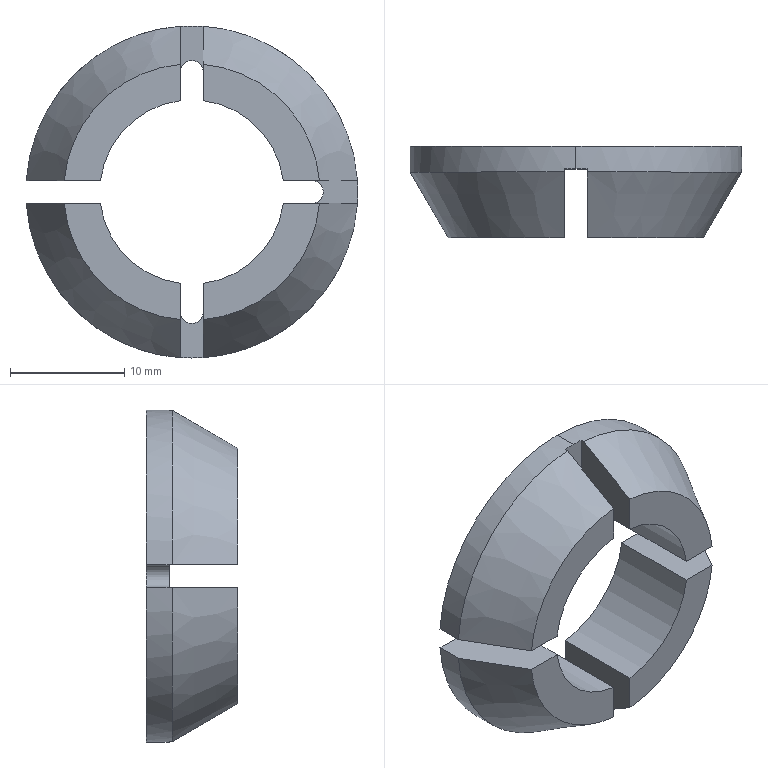Part | SolidWorks | features BaseBody 1 | 1 solid | 31 faces | box 29.013 x 8 x 29.047 mm | volume 2569 mm3 | plane 16 | cylinder 11 | cone 4 | commonest cylinder face diameters 16.12 x5 2 x3 29.047 x3
STEP:
#1=CARTESIAN_POINT('',(609.962,114.75,16.783));
#2=VERTEX_POINT('',#1);
#3=CARTESIAN_POINT('',(624.451,114.75,3.26));
#4=VERTEX_POINT('',#3);
#5=CARTESIAN_POINT('',(624.451,114.75,17.783));
#6=DIRECTION('',(0.,-1.,0.));
#7=DIRECTION('',(0.,0.,-1.));
#8=AXIS2_PLACEMENT_3D('',#5,#6,#7);
#9=CIRCLE('',#8,14.524);
#10=EDGE_CURVE('',#2,#4,#9,.T.);
#11=ORIENTED_EDGE('',*,*,#10,.T.);
#12=CARTESIAN_POINT('',(624.451,112.75,3.26));
#13=VERTEX_POINT('',#12);
#14=CARTESIAN_POINT('',(624.451,338.25,3.26));
#15=DIRECTION('',(0.,-1.,0.));
#16=VECTOR('',#15,1000.);
#17=LINE('',#14,#16);
#18=EDGE_CURVE('',#4,#13,#17,.T.);
#19=ORIENTED_EDGE('',*,*,#18,.T.);
#20=CARTESIAN_POINT('',(623.451,112.75,3.294));
#21=VERTEX_POINT('',#20);
#22=CARTESIAN_POINT('',(624.451,112.75,17.783));
#23=DIRECTION('',(0.,-1.,0.));
#24=DIRECTION('',(0.,0.,1.));
#25=AXIS2_PLACEMENT_3D('',#22,#23,#24);
#26=CIRCLE('',#25,14.524);
#27=EDGE_CURVE('',#21,#13,#26,.T.);
#28=ORIENTED_EDGE('',*,*,#27,.F.);
#29=CARTESIAN_POINT('',(623.451,112.482,3.294));
#30=VERTEX_POINT('',#29);
#31=CARTESIAN_POINT('',(623.451,112.482,3.294));
#32=DIRECTION('',(0.,1.,0.));
#33=VECTOR('',#32,1000.);
#34=LINE('',#31,#33);
#35=EDGE_CURVE('',#30,#21,#34,.T.);
#36=ORIENTED_EDGE('',*,*,#35,.F.);
#37=CARTESIAN_POINT('',(609.962,112.482,16.783));
#38=VERTEX_POINT('',#37);
#39=CARTESIAN_POINT('',(624.451,112.482,17.783));
#40=DIRECTION('',(0.,1.,0.));
#41=DIRECTION('',(0.,0.,1.));
#42=AXIS2_PLACEMENT_3D('',#39,#40,#41);
#43=CIRCLE('',#42,14.524);
#44=EDGE_CURVE('',#30,#38,#43,.T.);
#45=ORIENTED_EDGE('',*,*,#44,.T.);
#46=CARTESIAN_POINT('',(609.962,114.75,16.783));
#47=DIRECTION('',(0.,-1.,0.));
#48=VECTOR('',#47,1000.);
#49=LINE('',#46,#48);
#50=EDGE_CURVE('',#2,#38,#49,.T.);
#51=ORIENTED_EDGE('',*,*,#50,.F.);
#52=EDGE_LOOP('',(#11,#19,#28,#36,#45,#51));
#53=FACE_OUTER_BOUND('',#52,.T.);
#54=CARTESIAN_POINT('',(624.451,338.25,17.783));
#55=DIRECTION('',(0.,-1.,0.));
#56=DIRECTION('',(0.,0.,1.));
#57=AXIS2_PLACEMENT_3D('',#54,#55,#56);
#58=CYLINDRICAL_SURFACE('',#57,14.524);
#59=ADVANCED_FACE('',(#53),#58,.T.);
#60=ORIENTED_EDGE('',*,*,#18,.F.);
#61=CARTESIAN_POINT('',(624.451,114.75,32.307));
#62=VERTEX_POINT('',#61);
#63=CARTESIAN_POINT('',(624.451,114.75,17.783));
#64=DIRECTION('',(0.,-1.,0.));
#65=DIRECTION('',(0.,0.,-1.));
#66=AXIS2_PLACEMENT_3D('',#63,#64,#65);
#67=CIRCLE('',#66,14.524);
#68=EDGE_CURVE('',#4,#62,#67,.T.);
#69=ORIENTED_EDGE('',*,*,#68,.T.);
#70=CARTESIAN_POINT('',(624.451,112.75,32.307));
#71=VERTEX_POINT('',#70);
#72=CARTESIAN_POINT('',(624.451,338.25,32.307));
#73=DIRECTION('',(0.,-1.,0.));
#74=VECTOR('',#73,1000.);
#75=LINE('',#72,#74);
#76=EDGE_CURVE('',#62,#71,#75,.T.);
#77=ORIENTED_EDGE('',*,*,#76,.T.);
#78=CARTESIAN_POINT('',(625.451,112.75,32.273));
#79=VERTEX_POINT('',#78);
#80=CARTESIAN_POINT('',(624.451,112.75,17.783));
#81=DIRECTION('',(0.,-1.,0.));
#82=DIRECTION('',(0.,0.,1.));
#83=AXIS2_PLACEMENT_3D('',#80,#81,#82);
#84=CIRCLE('',#83,14.524);
#85=EDGE_CURVE('',#79,#71,#84,.T.);
#86=ORIENTED_EDGE('',*,*,#85,.F.);
#87=CARTESIAN_POINT('',(625.451,112.482,32.273));
#88=VERTEX_POINT('',#87);
#89=CARTESIAN_POINT('',(625.451,112.482,32.273));
#90=DIRECTION('',(0.,1.,0.));
#91=VECTOR('',#90,1000.);
#92=LINE('',#89,#91);
#93=EDGE_CURVE('',#88,#79,#92,.T.);
#94=ORIENTED_EDGE('',*,*,#93,.F.);
#95=CARTESIAN_POINT('',(638.94,112.482,18.783));
#96=VERTEX_POINT('',#95);
#97=CARTESIAN_POINT('',(624.451,112.482,17.783));
#98=DIRECTION('',(0.,1.,0.));
#99=DIRECTION('',(0.,0.,1.));
#100=AXIS2_PLACEMENT_3D('',#97,#98,#99);
#101=CIRCLE('',#100,14.524);
#102=EDGE_CURVE('',#88,#96,#101,.T.);
#103=ORIENTED_EDGE('',*,*,#102,.T.);
#104=CARTESIAN_POINT('',(638.94,112.75,18.783));
#105=VERTEX_POINT('',#104);
#106=CARTESIAN_POINT('',(638.94,112.75,18.783));
#107=DIRECTION('',(0.,-1.,0.));
#108=VECTOR('',#107,1000.);
#109=LINE('',#106,#108);
#110=EDGE_CURVE('',#105,#96,#109,.T.);
#111=ORIENTED_EDGE('',*,*,#110,.F.);
#112=CARTESIAN_POINT('',(638.94,112.75,16.783));
#113=VERTEX_POINT('',#112);
#114=CARTESIAN_POINT('',(624.451,112.75,17.783));
#115=DIRECTION('',(0.,-1.,0.));
#116=DIRECTION('',(0.,0.,1.));
#117=AXIS2_PLACEMENT_3D('',#114,#115,#116);
#118=CIRCLE('',#117,14.524);
#119=EDGE_CURVE('',#113,#105,#118,.T.);
#120=ORIENTED_EDGE('',*,*,#119,.F.);
#121=CARTESIAN_POINT('',(638.94,112.482,16.783));
#122=VERTEX_POINT('',#121);
#123=CARTESIAN_POINT('',(638.94,112.482,16.783));
#124=DIRECTION('',(0.,1.,0.));
#125=VECTOR('',#124,1000.);
#126=LINE('',#123,#125);
#127=EDGE_CURVE('',#122,#113,#126,.T.);
#128=ORIENTED_EDGE('',*,*,#127,.F.);
#129=CARTESIAN_POINT('',(625.451,112.482,3.294));
#130=VERTEX_POINT('',#129);
#131=CARTESIAN_POINT('',(624.451,112.482,17.783));
#132=DIRECTION('',(0.,1.,0.));
#133=DIRECTION('',(0.,0.,1.));
#134=AXIS2_PLACEMENT_3D('',#131,#132,#133);
#135=CIRCLE('',#134,14.524);
#136=EDGE_CURVE('',#122,#130,#135,.T.);
#137=ORIENTED_EDGE('',*,*,#136,.T.);
#138=CARTESIAN_POINT('',(625.451,112.75,3.294));
#139=VERTEX_POINT('',#138);
#140=CARTESIAN_POINT('',(625.451,112.75,3.294));
#141=DIRECTION('',(0.,-1.,0.));
#142=VECTOR('',#141,1000.);
#143=LINE('',#140,#142);
#144=EDGE_CURVE('',#139,#130,#143,.T.);
#145=ORIENTED_EDGE('',*,*,#144,.F.);
#146=CARTESIAN_POINT('',(624.451,112.75,17.783));
#147=DIRECTION('',(0.,-1.,0.));
#148=DIRECTION('',(0.,0.,1.));
#149=AXIS2_PLACEMENT_3D('',#146,#147,#148);
#150=CIRCLE('',#149,14.524);
#151=EDGE_CURVE('',#13,#139,#150,.T.);
#152=ORIENTED_EDGE('',*,*,#151,.F.);
#153=EDGE_LOOP('',(#60,#69,#77,#86,#94,#103,#111,#120,#128,#137,#145,#152));
#154=FACE_OUTER_BOUND('',#153,.T.);
#155=CARTESIAN_POINT('',(624.451,338.25,17.783));
#156=DIRECTION('',(0.,-1.,0.));
#157=DIRECTION('',(0.,0.,1.));
#158=AXIS2_PLACEMENT_3D('',#155,#156,#157);
#159=CYLINDRICAL_SURFACE('',#158,14.524);
#160=ADVANCED_FACE('',(#154),#159,.T.);
#161=CARTESIAN_POINT('',(619.27,114.75,11.609));
#162=VERTEX_POINT('',#161);
#163=CARTESIAN_POINT('',(623.451,114.75,9.786));
#164=VERTEX_POINT('',#163);
#165=CARTESIAN_POINT('',(624.451,114.75,17.783));
#166=DIRECTION('',(0.,-1.,0.));
#167=DIRECTION('',(0.,0.,-1.));
#168=AXIS2_PLACEMENT_3D('',#165,#166,#167);
#169=CIRCLE('',#168,8.06);
#170=EDGE_CURVE('',#162,#164,#169,.T.);
#171=ORIENTED_EDGE('',*,*,#170,.F.);
#172=CARTESIAN_POINT('',(619.27,106.75,11.609));
#173=VERTEX_POINT('',#172);
#174=CARTESIAN_POINT('',(619.27,110.25,11.609));
#175=DIRECTION('',(0.,-1.,0.));
#176=VECTOR('',#175,1000.);
#177=LINE('',#174,#176);
#178=EDGE_CURVE('',#162,#173,#177,.T.);
#179=ORIENTED_EDGE('',*,*,#178,.T.);
#180=CARTESIAN_POINT('',(623.451,106.75,9.786));
#181=VERTEX_POINT('',#180);
#182=CARTESIAN_POINT('',(624.451,106.75,17.783));
#183=DIRECTION('',(0.,-1.,0.));
#184=DIRECTION('',(0.,0.,-1.));
#185=AXIS2_PLACEMENT_3D('',#182,#183,#184);
#186=CIRCLE('',#185,8.06);
#187=EDGE_CURVE('',#173,#181,#186,.T.);
#188=ORIENTED_EDGE('',*,*,#187,.T.);
#189=CARTESIAN_POINT('',(623.451,110.25,9.786));
#190=DIRECTION('',(0.,1.,0.));
#191=VECTOR('',#190,1000.);
#192=LINE('',#189,#191);
#193=EDGE_CURVE('',#181,#164,#192,.T.);
#194=ORIENTED_EDGE('',*,*,#193,.T.);
#195=EDGE_LOOP('',(#171,#179,#188,#194));
#196=FACE_OUTER_BOUND('',#195,.T.);
#197=CARTESIAN_POINT('',(624.451,110.25,17.783));
#198=DIRECTION('',(0.,-1.,0.));
#199=DIRECTION('',(-0.6428,0.,-0.766));
#200=AXIS2_PLACEMENT_3D('',#197,#198,#199);
#201=CYLINDRICAL_SURFACE('',#200,8.06);
#202=ADVANCED_FACE('',(#196),#201,.F.);
#203=CARTESIAN_POINT('',(634.951,114.75,16.783));
#204=VERTEX_POINT('',#203);
#205=CARTESIAN_POINT('',(634.951,112.75,16.783));
#206=VERTEX_POINT('',#205);
#207=CARTESIAN_POINT('',(634.951,118.75,16.783));
#208=DIRECTION('',(0.,-1.,0.));
#209=VECTOR('',#208,1000.);
#210=LINE('',#207,#209);
#211=EDGE_CURVE('',#204,#206,#210,.T.);
#212=ORIENTED_EDGE('',*,*,#211,.T.);
#213=CARTESIAN_POINT('',(634.951,112.75,18.783));
#214=VERTEX_POINT('',#213);
#215=CARTESIAN_POINT('',(634.951,112.75,17.783));
#216=DIRECTION('',(0.,1.,0.));
#217=DIRECTION('',(0.,0.,1.));
#218=AXIS2_PLACEMENT_3D('',#215,#216,#217);
#219=CIRCLE('',#218,1.);
#220=EDGE_CURVE('',#214,#206,#219,.T.);
#221=ORIENTED_EDGE('',*,*,#220,.F.);
#222=CARTESIAN_POINT('',(634.951,114.75,18.783));
#223=VERTEX_POINT('',#222);
#224=CARTESIAN_POINT('',(634.951,118.75,18.783));
#225=DIRECTION('',(0.,1.,0.));
#226=VECTOR('',#225,1000.);
#227=LINE('',#224,#226);
#228=EDGE_CURVE('',#214,#223,#227,.T.);
#229=ORIENTED_EDGE('',*,*,#228,.T.);
#230=CARTESIAN_POINT('',(634.951,114.75,17.783));
#231=DIRECTION('',(0.,-1.,0.));
#232=DIRECTION('',(0.,0.,-1.));
#233=AXIS2_PLACEMENT_3D('',#230,#231,#232);
#234=CIRCLE('',#233,1.);
#235=EDGE_CURVE('',#204,#223,#234,.T.);
#236=ORIENTED_EDGE('',*,*,#235,.F.);
#237=EDGE_LOOP('',(#212,#221,#229,#236));
#238=FACE_OUTER_BOUND('',#237,.T.);
#239=CARTESIAN_POINT('',(634.951,118.75,17.783));
#240=DIRECTION('',(0.,-1.,0.));
#241=DIRECTION('',(0.,0.,1.));
#242=AXIS2_PLACEMENT_3D('',#239,#240,#241);
#243=CYLINDRICAL_SURFACE('',#242,1.);
#244=ADVANCED_FACE('',(#238),#243,.F.);
#245=CARTESIAN_POINT('',(623.451,114.75,7.283));
#246=VERTEX_POINT('',#245);
#247=CARTESIAN_POINT('',(623.451,112.75,7.283));
#248=VERTEX_POINT('',#247);
#249=CARTESIAN_POINT('',(623.451,118.75,7.283));
#250=DIRECTION('',(0.,-1.,0.));
#251=VECTOR('',#250,1000.);
#252=LINE('',#249,#251);
#253=EDGE_CURVE('',#246,#248,#252,.T.);
#254=ORIENTED_EDGE('',*,*,#253,.T.);
#255=CARTESIAN_POINT('',(625.451,112.75,7.283));
#256=VERTEX_POINT('',#255);
#257=CARTESIAN_POINT('',(624.451,112.75,7.283));
#258=DIRECTION('',(0.,1.,0.));
#259=DIRECTION('',(0.,0.,1.));
#260=AXIS2_PLACEMENT_3D('',#257,#258,#259);
#261=CIRCLE('',#260,1.);
#262=EDGE_CURVE('',#256,#248,#261,.T.);
#263=ORIENTED_EDGE('',*,*,#262,.F.);
#264=CARTESIAN_POINT('',(625.451,114.75,7.283));
#265=VERTEX_POINT('',#264);
#266=CARTESIAN_POINT('',(625.451,118.75,7.283));
#267=DIRECTION('',(0.,1.,0.));
#268=VECTOR('',#267,1000.);
#269=LINE('',#266,#268);
#270=EDGE_CURVE('',#256,#265,#269,.T.);
#271=ORIENTED_EDGE('',*,*,#270,.T.);
#272=CARTESIAN_POINT('',(624.451,114.75,7.283));
#273=DIRECTION('',(0.,-1.,0.));
#274=DIRECTION('',(0.,0.,-1.));
#275=AXIS2_PLACEMENT_3D('',#272,#273,#274);
#276=CIRCLE('',#275,1.);
#277=EDGE_CURVE('',#246,#265,#276,.T.);
#278=ORIENTED_EDGE('',*,*,#277,.F.);
#279=EDGE_LOOP('',(#254,#263,#271,#278));
#280=FACE_OUTER_BOUND('',#279,.T.);
#281=CARTESIAN_POINT('',(624.451,118.75,7.283));
#282=DIRECTION('',(0.,-1.,0.));
#283=DIRECTION('',(-1.,0.,0.));
#284=AXIS2_PLACEMENT_3D('',#281,#282,#283);
#285=CYLINDRICAL_SURFACE('',#284,1.);
#286=ADVANCED_FACE('',(#280),#285,.F.);
#287=CARTESIAN_POINT('',(625.451,114.75,28.283));
#288=VERTEX_POINT('',#287);
#289=CARTESIAN_POINT('',(625.451,112.75,28.283));
#290=VERTEX_POINT('',#289);
#291=CARTESIAN_POINT('',(625.451,118.75,28.283));
#292=DIRECTION('',(0.,-1.,0.));
#293=VECTOR('',#292,1000.);
#294=LINE('',#291,#293);
#295=EDGE_CURVE('',#288,#290,#294,.T.);
#296=ORIENTED_EDGE('',*,*,#295,.T.);
#297=CARTESIAN_POINT('',(623.451,112.75,28.283));
#298=VERTEX_POINT('',#297);
#299=CARTESIAN_POINT('',(624.451,112.75,28.283));
#300=DIRECTION('',(0.,1.,0.));
#301=DIRECTION('',(0.,0.,1.));
#302=AXIS2_PLACEMENT_3D('',#299,#300,#301);
#303=CIRCLE('',#302,1.);
#304=EDGE_CURVE('',#298,#290,#303,.T.);
#305=ORIENTED_EDGE('',*,*,#304,.F.);
#306=CARTESIAN_POINT('',(623.451,114.75,28.283));
#307=VERTEX_POINT('',#306);
#308=CARTESIAN_POINT('',(623.451,118.75,28.283));
#309=DIRECTION('',(0.,1.,0.));
#310=VECTOR('',#309,1000.);
#311=LINE('',#308,#310);
#312=EDGE_CURVE('',#298,#307,#311,.T.);
#313=ORIENTED_EDGE('',*,*,#312,.T.);
#314=CARTESIAN_POINT('',(624.451,114.75,28.283));
#315=DIRECTION('',(0.,-1.,0.));
#316=DIRECTION('',(0.,0.,-1.));
#317=AXIS2_PLACEMENT_3D('',#314,#315,#316);
#318=CIRCLE('',#317,1.);
#319=EDGE_CURVE('',#288,#307,#318,.T.);
#320=ORIENTED_EDGE('',*,*,#319,.F.);
#321=EDGE_LOOP('',(#296,#305,#313,#320));
#322=FACE_OUTER_BOUND('',#321,.T.);
#323=CARTESIAN_POINT('',(624.451,118.75,28.283));
#324=DIRECTION('',(0.,-1.,0.));
#325=DIRECTION('',(-1.,0.,0.));
#326=AXIS2_PLACEMENT_3D('',#323,#324,#325);
#327=CYLINDRICAL_SURFACE('',#326,1.);
#328=ADVANCED_FACE('',(#322),#327,.F.);
#329=CARTESIAN_POINT('',(613.282,106.75,16.783));
#330=VERTEX_POINT('',#329);
#331=CARTESIAN_POINT('',(616.453,106.75,16.783));
#332=VERTEX_POINT('',#331);
#333=CARTESIAN_POINT('',(624.451,106.75,16.783));
#334=DIRECTION('',(1.,0.,0.));
#335=VECTOR('',#334,1000.);
#336=LINE('',#333,#335);
#337=EDGE_CURVE('',#330,#332,#336,.T.);
#338=ORIENTED_EDGE('',*,*,#337,.T.);
#339=CARTESIAN_POINT('',(616.453,114.75,16.783));
#340=VERTEX_POINT('',#339);
#341=CARTESIAN_POINT('',(616.453,110.25,16.783));
#342=DIRECTION('',(0.,-1.,0.));
#343=VECTOR('',#342,1000.);
#344=LINE('',#341,#343);
#345=EDGE_CURVE('',#340,#332,#344,.T.);
#346=ORIENTED_EDGE('',*,*,#345,.F.);
#347=CARTESIAN_POINT('',(624.451,114.75,16.783));
#348=DIRECTION('',(1.,0.,0.));
#349=VECTOR('',#348,1000.);
#350=LINE('',#347,#349);
#351=EDGE_CURVE('',#2,#340,#350,.T.);
#352=ORIENTED_EDGE('',*,*,#351,.F.);
#353=ORIENTED_EDGE('',*,*,#50,.T.);
#354=CARTESIAN_POINT('',(613.282,106.75,16.783));
#355=CARTESIAN_POINT('',(612.174,108.66,16.783));
#356=CARTESIAN_POINT('',(611.068,110.571,16.783));
#357=CARTESIAN_POINT('',(609.962,112.482,16.783));
#358=B_SPLINE_CURVE_WITH_KNOTS('',3,(#354,#355,#356,#357),.UNSPECIFIED.,.F.,.F.,(4,4),(0.,1.),.UNSPECIFIED.);
#359=EDGE_CURVE('',#330,#38,#358,.T.);
#360=ORIENTED_EDGE('',*,*,#359,.F.);
#361=EDGE_LOOP('',(#338,#346,#352,#353,#360));
#362=FACE_OUTER_BOUND('',#361,.T.);
#363=CARTESIAN_POINT('',(624.451,111.75,16.783));
#364=DIRECTION('',(0.,0.,-1.));
#365=DIRECTION('',(-1.,0.,0.));
#366=AXIS2_PLACEMENT_3D('',#363,#364,#365);
#367=PLANE('',#366);
#368=ADVANCED_FACE('',(#362),#367,.F.);
#369=CARTESIAN_POINT('',(616.453,106.75,18.783));
#370=VERTEX_POINT('',#369);
#371=CARTESIAN_POINT('',(616.453,114.75,18.783));
#372=VERTEX_POINT('',#371);
#373=CARTESIAN_POINT('',(616.453,110.25,18.783));
#374=DIRECTION('',(0.,1.,0.));
#375=VECTOR('',#374,1000.);
#376=LINE('',#373,#375);
#377=EDGE_CURVE('',#370,#372,#376,.T.);
#378=ORIENTED_EDGE('',*,*,#377,.F.);
#379=CARTESIAN_POINT('',(613.282,106.75,18.783));
#380=VERTEX_POINT('',#379);
#381=CARTESIAN_POINT('',(624.451,106.75,18.783));
#382=DIRECTION('',(-1.,0.,0.));
#383=VECTOR('',#382,1000.);
#384=LINE('',#381,#383);
#385=EDGE_CURVE('',#370,#380,#384,.T.);
#386=ORIENTED_EDGE('',*,*,#385,.T.);
#387=CARTESIAN_POINT('',(609.962,112.482,18.783));
#388=VERTEX_POINT('',#387);
#389=CARTESIAN_POINT('',(609.962,112.482,18.783));
#390=CARTESIAN_POINT('',(611.068,110.571,18.783));
#391=CARTESIAN_POINT('',(612.174,108.66,18.783));
#392=CARTESIAN_POINT('',(613.282,106.75,18.783));
#393=B_SPLINE_CURVE_WITH_KNOTS('',3,(#389,#390,#391,#392),.UNSPECIFIED.,.F.,.F.,(4,4),(0.,1.),.UNSPECIFIED.);
#394=EDGE_CURVE('',#388,#380,#393,.T.);
#395=ORIENTED_EDGE('',*,*,#394,.F.);
#396=CARTESIAN_POINT('',(609.962,114.75,18.783));
#397=VERTEX_POINT('',#396);
#398=CARTESIAN_POINT('',(609.962,338.25,18.783));
#399=DIRECTION('',(0.,1.,0.));
#400=VECTOR('',#399,1000.);
#401=LINE('',#398,#400);
#402=EDGE_CURVE('',#388,#397,#401,.T.);
#403=ORIENTED_EDGE('',*,*,#402,.T.);
#404=CARTESIAN_POINT('',(624.451,114.75,18.783));
#405=DIRECTION('',(-1.,0.,0.));
#406=VECTOR('',#405,1000.);
#407=LINE('',#404,#406);
#408=EDGE_CURVE('',#372,#397,#407,.T.);
#409=ORIENTED_EDGE('',*,*,#408,.F.);
#410=EDGE_LOOP('',(#378,#386,#395,#403,#409));
#411=FACE_OUTER_BOUND('',#410,.T.);
#412=CARTESIAN_POINT('',(624.451,111.75,18.783));
#413=DIRECTION('',(0.,0.,1.));
#414=DIRECTION('',(0.,-1.,0.));
#415=AXIS2_PLACEMENT_3D('',#412,#413,#414);
#416=PLANE('',#415);
#417=ADVANCED_FACE('',(#411),#416,.F.);
#418=CARTESIAN_POINT('',(625.451,106.75,25.781));
#419=VERTEX_POINT('',#418);
#420=CARTESIAN_POINT('',(625.451,106.75,28.953));
#421=VERTEX_POINT('',#420);
#422=CARTESIAN_POINT('',(625.451,106.75,17.783));
#423=DIRECTION('',(0.,0.,1.));
#424=VECTOR('',#423,1000.);
#425=LINE('',#422,#424);
#426=EDGE_CURVE('',#419,#421,#425,.T.);
#427=ORIENTED_EDGE('',*,*,#426,.F.);
#428=CARTESIAN_POINT('',(632.449,106.75,18.783));
#429=VERTEX_POINT('',#428);
#430=CARTESIAN_POINT('',(624.451,106.75,17.783));
#431=DIRECTION('',(0.,-1.,0.));
#432=DIRECTION('',(0.,0.,-1.));
#433=AXIS2_PLACEMENT_3D('',#430,#431,#432);
#434=CIRCLE('',#433,8.06);
#435=EDGE_CURVE('',#429,#419,#434,.T.);
#436=ORIENTED_EDGE('',*,*,#435,.F.);
#437=CARTESIAN_POINT('',(635.62,106.75,18.783));
#438=VERTEX_POINT('',#437);
#439=CARTESIAN_POINT('',(624.451,106.75,18.783));
#440=DIRECTION('',(-1.,0.,0.));
#441=VECTOR('',#440,1000.);
#442=LINE('',#439,#441);
#443=EDGE_CURVE('',#438,#429,#442,.T.);
#444=ORIENTED_EDGE('',*,*,#443,.F.);
#445=CARTESIAN_POINT('',(624.451,106.75,17.783));
#446=DIRECTION('',(0.,-1.,0.));
#447=DIRECTION('',(0.,0.,-1.));
#448=AXIS2_PLACEMENT_3D('',#445,#446,#447);
#449=CIRCLE('',#448,11.214);
#450=EDGE_CURVE('',#438,#421,#449,.T.);
#451=ORIENTED_EDGE('',*,*,#450,.T.);
#452=EDGE_LOOP('',(#427,#436,#444,#451));
#453=FACE_OUTER_BOUND('',#452,.T.);
#454=CARTESIAN_POINT('',(624.451,106.75,17.783));
#455=DIRECTION('',(0.,-1.,0.));
#456=DIRECTION('',(0.,0.,-1.));
#457=AXIS2_PLACEMENT_3D('',#454,#455,#456);
#458=PLANE('',#457);
#459=ADVANCED_FACE('',(#453),#458,.T.);
#460=ORIENTED_EDGE('',*,*,#385,.F.);
#461=CARTESIAN_POINT('',(623.451,106.75,25.781));
#462=VERTEX_POINT('',#461);
#463=CARTESIAN_POINT('',(624.451,106.75,17.783));
#464=DIRECTION('',(0.,-1.,0.));
#465=DIRECTION('',(0.,0.,-1.));
#466=AXIS2_PLACEMENT_3D('',#463,#464,#465);
#467=CIRCLE('',#466,8.06);
#468=EDGE_CURVE('',#462,#370,#467,.T.);
#469=ORIENTED_EDGE('',*,*,#468,.F.);
#470=CARTESIAN_POINT('',(623.451,106.75,28.953));
#471=VERTEX_POINT('',#470);
#472=CARTESIAN_POINT('',(623.451,106.75,17.783));
#473=DIRECTION('',(0.,0.,-1.));
#474=VECTOR('',#473,1000.);
#475=LINE('',#472,#474);
#476=EDGE_CURVE('',#471,#462,#475,.T.);
#477=ORIENTED_EDGE('',*,*,#476,.F.);
#478=CARTESIAN_POINT('',(624.451,106.75,17.783));
#479=DIRECTION('',(0.,-1.,0.));
#480=DIRECTION('',(0.,0.,-1.));
#481=AXIS2_PLACEMENT_3D('',#478,#479,#480);
#482=CIRCLE('',#481,11.214);
#483=EDGE_CURVE('',#471,#380,#482,.T.);
#484=ORIENTED_EDGE('',*,*,#483,.T.);
#485=EDGE_LOOP('',(#460,#469,#477,#484));
#486=FACE_OUTER_BOUND('',#485,.T.);
#487=CARTESIAN_POINT('',(624.451,106.75,17.783));
#488=DIRECTION('',(0.,-1.,0.));
#489=DIRECTION('',(0.,0.,-1.));
#490=AXIS2_PLACEMENT_3D('',#487,#488,#489);
#491=PLANE('',#490);
#492=ADVANCED_FACE('',(#486),#491,.T.);
#493=CARTESIAN_POINT('',(623.451,106.75,6.614));
#494=VERTEX_POINT('',#493);
#495=CARTESIAN_POINT('',(623.451,106.75,17.783));
#496=DIRECTION('',(0.,0.,-1.));
#497=VECTOR('',#496,1000.);
#498=LINE('',#495,#497);
#499=EDGE_CURVE('',#181,#494,#498,.T.);
#500=ORIENTED_EDGE('',*,*,#499,.F.);
#501=ORIENTED_EDGE('',*,*,#187,.F.);
#502=CARTESIAN_POINT('',(624.451,106.75,17.783));
#503=DIRECTION('',(0.,-1.,0.));
#504=DIRECTION('',(0.,0.,-1.));
#505=AXIS2_PLACEMENT_3D('',#502,#503,#504);
#506=CIRCLE('',#505,8.06);
#507=EDGE_CURVE('',#332,#173,#506,.T.);
#508=ORIENTED_EDGE('',*,*,#507,.F.);
#509=ORIENTED_EDGE('',*,*,#337,.F.);
#510=CARTESIAN_POINT('',(624.451,106.75,17.783));
#511=DIRECTION('',(0.,-1.,0.));
#512=DIRECTION('',(0.,0.,-1.));
#513=AXIS2_PLACEMENT_3D('',#510,#511,#512);
#514=CIRCLE('',#513,11.214);
#515=EDGE_CURVE('',#330,#494,#514,.T.);
#516=ORIENTED_EDGE('',*,*,#515,.T.);
#517=EDGE_LOOP('',(#500,#501,#508,#509,#516));
#518=FACE_OUTER_BOUND('',#517,.T.);
#519=CARTESIAN_POINT('',(624.451,106.75,17.783));
#520=DIRECTION('',(0.,-1.,0.));
#521=DIRECTION('',(0.,0.,-1.));
#522=AXIS2_PLACEMENT_3D('',#519,#520,#521);
#523=PLANE('',#522);
#524=ADVANCED_FACE('',(#518),#523,.T.);
#525=CARTESIAN_POINT('',(632.449,106.75,16.783));
#526=VERTEX_POINT('',#525);
#527=CARTESIAN_POINT('',(635.62,106.75,16.783));
#528=VERTEX_POINT('',#527);
#529=CARTESIAN_POINT('',(624.451,106.75,16.783));
#530=DIRECTION('',(1.,0.,0.));
#531=VECTOR('',#530,1000.);
#532=LINE('',#529,#531);
#533=EDGE_CURVE('',#526,#528,#532,.T.);
#534=ORIENTED_EDGE('',*,*,#533,.F.);
#535=CARTESIAN_POINT('',(625.451,106.75,9.786));
#536=VERTEX_POINT('',#535);
#537=CARTESIAN_POINT('',(624.451,106.75,17.783));
#538=DIRECTION('',(0.,-1.,0.));
#539=DIRECTION('',(0.,0.,-1.));
#540=AXIS2_PLACEMENT_3D('',#537,#538,#539);
#541=CIRCLE('',#540,8.06);
#542=EDGE_CURVE('',#536,#526,#541,.T.);
#543=ORIENTED_EDGE('',*,*,#542,.F.);
#544=CARTESIAN_POINT('',(625.451,106.75,6.614));
#545=VERTEX_POINT('',#544);
#546=CARTESIAN_POINT('',(625.451,106.75,17.783));
#547=DIRECTION('',(0.,0.,1.));
#548=VECTOR('',#547,1000.);
#549=LINE('',#546,#548);
#550=EDGE_CURVE('',#545,#536,#549,.T.);
#551=ORIENTED_EDGE('',*,*,#550,.F.);
#552=CARTESIAN_POINT('',(624.451,106.75,17.783));
#553=DIRECTION('',(0.,-1.,0.));
#554=DIRECTION('',(0.,0.,-1.));
#555=AXIS2_PLACEMENT_3D('',#552,#553,#554);
#556=CIRCLE('',#555,11.214);
#557=EDGE_CURVE('',#545,#528,#556,.T.);
#558=ORIENTED_EDGE('',*,*,#557,.T.);
#559=EDGE_LOOP('',(#534,#543,#551,#558));
#560=FACE_OUTER_BOUND('',#559,.T.);
#561=CARTESIAN_POINT('',(624.451,106.75,17.783));
#562=DIRECTION('',(0.,-1.,0.));
#563=DIRECTION('',(0.,0.,-1.));
#564=AXIS2_PLACEMENT_3D('',#561,#562,#563);
#565=PLANE('',#564);
#566=ADVANCED_FACE('',(#560),#565,.T.);
#567=CARTESIAN_POINT('',(625.451,112.482,32.273));
#568=CARTESIAN_POINT('',(625.451,110.571,31.167));
#569=CARTESIAN_POINT('',(625.451,108.66,30.06));
#570=CARTESIAN_POINT('',(625.451,106.75,28.953));
#571=B_SPLINE_CURVE_WITH_KNOTS('',3,(#567,#568,#569,#570),.UNSPECIFIED.,.F.,.F.,(4,4),(0.,1.),.UNSPECIFIED.);
#572=EDGE_CURVE('',#88,#421,#571,.T.);
#573=ORIENTED_EDGE('',*,*,#572,.T.);
#574=ORIENTED_EDGE('',*,*,#450,.F.);
#575=CARTESIAN_POINT('',(635.62,106.75,18.783));
#576=CARTESIAN_POINT('',(636.103,107.582,18.783));
#577=CARTESIAN_POINT('',(636.585,108.415,18.783));
#578=CARTESIAN_POINT('',(637.692,110.325,18.783));
#579=CARTESIAN_POINT('',(638.316,111.404,18.783));
#580=CARTESIAN_POINT('',(638.94,112.482,18.783));
#581=B_SPLINE_CURVE_WITH_KNOTS('',3,(#575,#576,#577,#578,#579,#580),.UNSPECIFIED.,.F.,.F.,(4,2,4),(0.,0.4357,1.),.UNSPECIFIED.);
#582=EDGE_CURVE('',#438,#96,#581,.T.);
#583=ORIENTED_EDGE('',*,*,#582,.T.);
#584=ORIENTED_EDGE('',*,*,#102,.F.);
#585=EDGE_LOOP('',(#573,#574,#583,#584));
#586=FACE_OUTER_BOUND('',#585,.T.);
#587=CARTESIAN_POINT('',(624.451,104.25,17.783));
#588=DIRECTION('',(0.,1.,0.));
#589=DIRECTION('',(0.,0.,-1.));
#590=AXIS2_PLACEMENT_3D('',#587,#588,#589);
#591=CONICAL_SURFACE('',#590,9.771,0.5236);
#592=ADVANCED_FACE('',(#586),#591,.T.);
#593=CARTESIAN_POINT('',(632.449,114.75,18.783));
#594=VERTEX_POINT('',#593);
#595=CARTESIAN_POINT('',(632.449,110.25,18.783));
#596=DIRECTION('',(0.,-1.,0.));
#597=VECTOR('',#596,1000.);
#598=LINE('',#595,#597);
#599=EDGE_CURVE('',#594,#429,#598,.T.);
#600=ORIENTED_EDGE('',*,*,#599,.T.);
#601=ORIENTED_EDGE('',*,*,#435,.T.);
#602=CARTESIAN_POINT('',(625.451,114.75,25.781));
#603=VERTEX_POINT('',#602);
#604=CARTESIAN_POINT('',(625.451,110.25,25.781));
#605=DIRECTION('',(0.,1.,0.));
#606=VECTOR('',#605,1000.);
#607=LINE('',#604,#606);
#608=EDGE_CURVE('',#419,#603,#607,.T.);
#609=ORIENTED_EDGE('',*,*,#608,.T.);
#610=CARTESIAN_POINT('',(624.451,114.75,17.783));
#611=DIRECTION('',(0.,-1.,0.));
#612=DIRECTION('',(0.,0.,-1.));
#613=AXIS2_PLACEMENT_3D('',#610,#611,#612);
#614=CIRCLE('',#613,8.06);
#615=EDGE_CURVE('',#594,#603,#614,.T.);
#616=ORIENTED_EDGE('',*,*,#615,.F.);
#617=EDGE_LOOP('',(#600,#601,#609,#616));
#618=FACE_OUTER_BOUND('',#617,.T.);
#619=CARTESIAN_POINT('',(624.451,110.25,17.783));
#620=DIRECTION('',(0.,-1.,0.));
#621=DIRECTION('',(-0.6428,0.,-0.766));
#622=AXIS2_PLACEMENT_3D('',#619,#620,#621);
#623=CYLINDRICAL_SURFACE('',#622,8.06);
#624=ADVANCED_FACE('',(#618),#623,.F.);
#625=ORIENTED_EDGE('',*,*,#394,.T.);
#626=ORIENTED_EDGE('',*,*,#483,.F.);
#627=CARTESIAN_POINT('',(623.451,112.482,32.273));
#628=VERTEX_POINT('',#627);
#629=CARTESIAN_POINT('',(623.451,106.75,28.953));
#630=CARTESIAN_POINT('',(623.451,107.582,29.435));
#631=CARTESIAN_POINT('',(623.451,108.415,29.918));
#632=CARTESIAN_POINT('',(623.451,110.325,31.024));
#633=CARTESIAN_POINT('',(623.451,111.404,31.648));
#634=CARTESIAN_POINT('',(623.451,112.482,32.273));
#635=B_SPLINE_CURVE_WITH_KNOTS('',3,(#629,#630,#631,#632,#633,#634),.UNSPECIFIED.,.F.,.F.,(4,2,4),(0.,0.4357,1.),.UNSPECIFIED.);
#636=EDGE_CURVE('',#471,#628,#635,.T.);
#637=ORIENTED_EDGE('',*,*,#636,.T.);
#638=CARTESIAN_POINT('',(624.451,112.482,17.783));
#639=DIRECTION('',(0.,1.,0.));
#640=DIRECTION('',(0.,0.,1.));
#641=AXIS2_PLACEMENT_3D('',#638,#639,#640);
#642=CIRCLE('',#641,14.524);
#643=EDGE_CURVE('',#388,#628,#642,.T.);
#644=ORIENTED_EDGE('',*,*,#643,.F.);
#645=EDGE_LOOP('',(#625,#626,#637,#644));
#646=FACE_OUTER_BOUND('',#645,.T.);
#647=CARTESIAN_POINT('',(624.451,104.25,17.783));
#648=DIRECTION('',(0.,1.,0.));
#649=DIRECTION('',(0.,0.,-1.));
#650=AXIS2_PLACEMENT_3D('',#647,#648,#649);
#651=CONICAL_SURFACE('',#650,9.771,0.5236);
#652=ADVANCED_FACE('',(#646),#651,.T.);
#653=CARTESIAN_POINT('',(623.451,112.482,3.294));
#654=CARTESIAN_POINT('',(623.451,110.571,4.4));
#655=CARTESIAN_POINT('',(623.451,108.66,5.507));
#656=CARTESIAN_POINT('',(623.451,106.75,6.614));
#657=B_SPLINE_CURVE_WITH_KNOTS('',3,(#653,#654,#655,#656),.UNSPECIFIED.,.F.,.F.,(4,4),(0.,1.),.UNSPECIFIED.);
#658=EDGE_CURVE('',#30,#494,#657,.T.);
#659=ORIENTED_EDGE('',*,*,#658,.T.);
#660=ORIENTED_EDGE('',*,*,#515,.F.);
#661=ORIENTED_EDGE('',*,*,#359,.T.);
#662=ORIENTED_EDGE('',*,*,#44,.F.);
#663=EDGE_LOOP('',(#659,#660,#661,#662));
#664=FACE_OUTER_BOUND('',#663,.T.);
#665=CARTESIAN_POINT('',(624.451,104.25,17.783));
#666=DIRECTION('',(0.,1.,0.));
#667=DIRECTION('',(0.,0.,-1.));
#668=AXIS2_PLACEMENT_3D('',#665,#666,#667);
#669=CONICAL_SURFACE('',#668,9.771,0.5236);
#670=ADVANCED_FACE('',(#664),#669,.T.);
#671=CARTESIAN_POINT('',(638.94,112.482,16.783));
#672=CARTESIAN_POINT('',(638.316,111.404,16.783));
#673=CARTESIAN_POINT('',(637.692,110.325,16.783));
#674=CARTESIAN_POINT('',(636.585,108.415,16.783));
#675=CARTESIAN_POINT('',(636.103,107.582,16.783));
#676=CARTESIAN_POINT('',(635.62,106.75,16.783));
#677=B_SPLINE_CURVE_WITH_KNOTS('',3,(#671,#672,#673,#674,#675,#676),.UNSPECIFIED.,.F.,.F.,(4,2,4),(0.,0.5643,1.),.UNSPECIFIED.);
#678=EDGE_CURVE('',#122,#528,#677,.T.);
#679=ORIENTED_EDGE('',*,*,#678,.T.);
#680=ORIENTED_EDGE('',*,*,#557,.F.);
#681=CARTESIAN_POINT('',(625.451,106.75,6.614));
#682=CARTESIAN_POINT('',(625.451,107.582,6.132));
#683=CARTESIAN_POINT('',(625.451,108.415,5.649));
#684=CARTESIAN_POINT('',(625.451,110.325,4.543));
#685=CARTESIAN_POINT('',(625.451,111.404,3.918));
#686=CARTESIAN_POINT('',(625.451,112.482,3.294));
#687=B_SPLINE_CURVE_WITH_KNOTS('',3,(#681,#682,#683,#684,#685,#686),.UNSPECIFIED.,.F.,.F.,(4,2,4),(0.,0.4357,1.),.UNSPECIFIED.);
#688=EDGE_CURVE('',#545,#130,#687,.T.);
#689=ORIENTED_EDGE('',*,*,#688,.T.);
#690=ORIENTED_EDGE('',*,*,#136,.F.);
#691=EDGE_LOOP('',(#679,#680,#689,#690));
#692=FACE_OUTER_BOUND('',#691,.T.);
#693=CARTESIAN_POINT('',(624.451,104.25,17.783));
#694=DIRECTION('',(0.,1.,0.));
#695=DIRECTION('',(0.,0.,-1.));
#696=AXIS2_PLACEMENT_3D('',#693,#694,#695);
#697=CONICAL_SURFACE('',#696,9.771,0.5236);
#698=ADVANCED_FACE('',(#692),#697,.T.);
#699=CARTESIAN_POINT('',(623.451,114.75,25.781));
#700=VERTEX_POINT('',#699);
#701=CARTESIAN_POINT('',(623.451,110.25,25.781));
#702=DIRECTION('',(0.,-1.,0.));
#703=VECTOR('',#702,1000.);
#704=LINE('',#701,#703);
#705=EDGE_CURVE('',#700,#462,#704,.T.);
#706=ORIENTED_EDGE('',*,*,#705,.T.);
#707=ORIENTED_EDGE('',*,*,#468,.T.);
#708=ORIENTED_EDGE('',*,*,#377,.T.);
#709=CARTESIAN_POINT('',(624.451,114.75,17.783));
#710=DIRECTION('',(0.,-1.,0.));
#711=DIRECTION('',(0.,0.,-1.));
#712=AXIS2_PLACEMENT_3D('',#709,#710,#711);
#713=CIRCLE('',#712,8.06);
#714=EDGE_CURVE('',#700,#372,#713,.T.);
#715=ORIENTED_EDGE('',*,*,#714,.F.);
#716=EDGE_LOOP('',(#706,#707,#708,#715));
#717=FACE_OUTER_BOUND('',#716,.T.);
#718=CARTESIAN_POINT('',(624.451,110.25,17.783));
#719=DIRECTION('',(0.,-1.,0.));
#720=DIRECTION('',(-0.6428,0.,-0.766));
#721=AXIS2_PLACEMENT_3D('',#718,#719,#720);
#722=CYLINDRICAL_SURFACE('',#721,8.06);
#723=ADVANCED_FACE('',(#717),#722,.F.);
#724=CARTESIAN_POINT('',(625.451,114.75,9.786));
#725=VERTEX_POINT('',#724);
#726=CARTESIAN_POINT('',(625.451,110.25,9.786));
#727=DIRECTION('',(0.,-1.,0.));
#728=VECTOR('',#727,1000.);
#729=LINE('',#726,#728);
#730=EDGE_CURVE('',#725,#536,#729,.T.);
#731=ORIENTED_EDGE('',*,*,#730,.T.);
#732=ORIENTED_EDGE('',*,*,#542,.T.);
#733=CARTESIAN_POINT('',(632.449,114.75,16.783));
#734=VERTEX_POINT('',#733);
#735=CARTESIAN_POINT('',(632.449,110.25,16.783));
#736=DIRECTION('',(0.,1.,0.));
#737=VECTOR('',#736,1000.);
#738=LINE('',#735,#737);
#739=EDGE_CURVE('',#526,#734,#738,.T.);
#740=ORIENTED_EDGE('',*,*,#739,.T.);
#741=CARTESIAN_POINT('',(624.451,114.75,17.783));
#742=DIRECTION('',(0.,-1.,0.));
#743=DIRECTION('',(0.,0.,-1.));
#744=AXIS2_PLACEMENT_3D('',#741,#742,#743);
#745=CIRCLE('',#744,8.06);
#746=EDGE_CURVE('',#725,#734,#745,.T.);
#747=ORIENTED_EDGE('',*,*,#746,.F.);
#748=EDGE_LOOP('',(#731,#732,#740,#747));
#749=FACE_OUTER_BOUND('',#748,.T.);
#750=CARTESIAN_POINT('',(624.451,110.25,17.783));
#751=DIRECTION('',(0.,-1.,0.));
#752=DIRECTION('',(-0.6428,0.,-0.766));
#753=AXIS2_PLACEMENT_3D('',#750,#751,#752);
#754=CYLINDRICAL_SURFACE('',#753,8.06);
#755=ADVANCED_FACE('',(#749),#754,.F.);
#756=ORIENTED_EDGE('',*,*,#85,.T.);
#757=CARTESIAN_POINT('',(623.451,112.75,32.273));
#758=VERTEX_POINT('',#757);
#759=CARTESIAN_POINT('',(624.451,112.75,17.783));
#760=DIRECTION('',(0.,-1.,0.));
#761=DIRECTION('',(0.,0.,1.));
#762=AXIS2_PLACEMENT_3D('',#759,#760,#761);
#763=CIRCLE('',#762,14.524);
#764=EDGE_CURVE('',#71,#758,#763,.T.);
#765=ORIENTED_EDGE('',*,*,#764,.T.);
#766=CARTESIAN_POINT('',(623.451,112.75,17.783));
#767=DIRECTION('',(0.,0.,-1.));
#768=VECTOR('',#767,1000.);
#769=LINE('',#766,#768);
#770=EDGE_CURVE('',#758,#298,#769,.T.);
#771=ORIENTED_EDGE('',*,*,#770,.T.);
#772=ORIENTED_EDGE('',*,*,#304,.T.);
#773=CARTESIAN_POINT('',(625.451,112.75,17.783));
#774=DIRECTION('',(0.,0.,1.));
#775=VECTOR('',#774,1000.);
#776=LINE('',#773,#775);
#777=EDGE_CURVE('',#290,#79,#776,.T.);
#778=ORIENTED_EDGE('',*,*,#777,.T.);
#779=EDGE_LOOP('',(#756,#765,#771,#772,#778));
#780=FACE_OUTER_BOUND('',#779,.T.);
#781=CARTESIAN_POINT('',(624.451,112.75,17.783));
#782=DIRECTION('',(0.,1.,0.));
#783=DIRECTION('',(0.,0.,-1.));
#784=AXIS2_PLACEMENT_3D('',#781,#782,#783);
#785=PLANE('',#784);
#786=ADVANCED_FACE('',(#780),#785,.F.);
#787=ORIENTED_EDGE('',*,*,#27,.T.);
#788=ORIENTED_EDGE('',*,*,#151,.T.);
#789=CARTESIAN_POINT('',(625.451,112.75,17.783));
#790=DIRECTION('',(0.,0.,1.));
#791=VECTOR('',#790,1000.);
#792=LINE('',#789,#791);
#793=EDGE_CURVE('',#139,#256,#792,.T.);
#794=ORIENTED_EDGE('',*,*,#793,.T.);
#795=ORIENTED_EDGE('',*,*,#262,.T.);
#796=CARTESIAN_POINT('',(623.451,112.75,17.783));
#797=DIRECTION('',(0.,0.,-1.));
#798=VECTOR('',#797,1000.);
#799=LINE('',#796,#798);
#800=EDGE_CURVE('',#248,#21,#799,.T.);
#801=ORIENTED_EDGE('',*,*,#800,.T.);
#802=EDGE_LOOP('',(#787,#788,#794,#795,#801));
#803=FACE_OUTER_BOUND('',#802,.T.);
#804=CARTESIAN_POINT('',(624.451,112.75,17.783));
#805=DIRECTION('',(0.,1.,0.));
#806=DIRECTION('',(0.,0.,-1.));
#807=AXIS2_PLACEMENT_3D('',#804,#805,#806);
#808=PLANE('',#807);
#809=ADVANCED_FACE('',(#803),#808,.F.);
#810=ORIENTED_EDGE('',*,*,#119,.T.);
#811=CARTESIAN_POINT('',(624.451,112.75,18.783));
#812=DIRECTION('',(-1.,0.,0.));
#813=VECTOR('',#812,1000.);
#814=LINE('',#811,#813);
#815=EDGE_CURVE('',#105,#214,#814,.T.);
#816=ORIENTED_EDGE('',*,*,#815,.T.);
#817=ORIENTED_EDGE('',*,*,#220,.T.);
#818=CARTESIAN_POINT('',(624.451,112.75,16.783));
#819=DIRECTION('',(1.,0.,0.));
#820=VECTOR('',#819,1000.);
#821=LINE('',#818,#820);
#822=EDGE_CURVE('',#206,#113,#821,.T.);
#823=ORIENTED_EDGE('',*,*,#822,.T.);
#824=EDGE_LOOP('',(#810,#816,#817,#823));
#825=FACE_OUTER_BOUND('',#824,.T.);
#826=CARTESIAN_POINT('',(624.451,112.75,17.783));
#827=DIRECTION('',(0.,1.,0.));
#828=DIRECTION('',(0.,0.,-1.));
#829=AXIS2_PLACEMENT_3D('',#826,#827,#828);
#830=PLANE('',#829);
#831=ADVANCED_FACE('',(#825),#830,.F.);
#832=CARTESIAN_POINT('',(624.451,114.75,16.783));
#833=DIRECTION('',(1.,0.,0.));
#834=VECTOR('',#833,1000.);
#835=LINE('',#832,#834);
#836=EDGE_CURVE('',#734,#204,#835,.T.);
#837=ORIENTED_EDGE('',*,*,#836,.T.);
#838=ORIENTED_EDGE('',*,*,#235,.T.);
#839=CARTESIAN_POINT('',(624.451,114.75,18.783));
#840=DIRECTION('',(-1.,0.,0.));
#841=VECTOR('',#840,1000.);
#842=LINE('',#839,#841);
#843=EDGE_CURVE('',#223,#594,#842,.T.);
#844=ORIENTED_EDGE('',*,*,#843,.T.);
#845=ORIENTED_EDGE('',*,*,#615,.T.);
#846=CARTESIAN_POINT('',(625.451,114.75,17.783));
#847=DIRECTION('',(0.,0.,1.));
#848=VECTOR('',#847,1000.);
#849=LINE('',#846,#848);
#850=EDGE_CURVE('',#603,#288,#849,.T.);
#851=ORIENTED_EDGE('',*,*,#850,.T.);
#852=ORIENTED_EDGE('',*,*,#319,.T.);
#853=CARTESIAN_POINT('',(623.451,114.75,17.783));
#854=DIRECTION('',(0.,0.,-1.));
#855=VECTOR('',#854,1000.);
#856=LINE('',#853,#855);
#857=EDGE_CURVE('',#307,#700,#856,.T.);
#858=ORIENTED_EDGE('',*,*,#857,.T.);
#859=ORIENTED_EDGE('',*,*,#714,.T.);
#860=ORIENTED_EDGE('',*,*,#408,.T.);
#861=CARTESIAN_POINT('',(624.451,114.75,17.783));
#862=DIRECTION('',(0.,-1.,0.));
#863=DIRECTION('',(0.,0.,-1.));
#864=AXIS2_PLACEMENT_3D('',#861,#862,#863);
#865=CIRCLE('',#864,14.524);
#866=EDGE_CURVE('',#62,#397,#865,.T.);
#867=ORIENTED_EDGE('',*,*,#866,.F.);
#868=ORIENTED_EDGE('',*,*,#68,.F.);
#869=ORIENTED_EDGE('',*,*,#10,.F.);
#870=ORIENTED_EDGE('',*,*,#351,.T.);
#871=CARTESIAN_POINT('',(624.451,114.75,17.783));
#872=DIRECTION('',(0.,-1.,0.));
#873=DIRECTION('',(0.,0.,-1.));
#874=AXIS2_PLACEMENT_3D('',#871,#872,#873);
#875=CIRCLE('',#874,8.06);
#876=EDGE_CURVE('',#340,#162,#875,.T.);
#877=ORIENTED_EDGE('',*,*,#876,.T.);
#878=ORIENTED_EDGE('',*,*,#170,.T.);
#879=CARTESIAN_POINT('',(623.451,114.75,17.783));
#880=DIRECTION('',(0.,0.,-1.));
#881=VECTOR('',#880,1000.);
#882=LINE('',#879,#881);
#883=EDGE_CURVE('',#164,#246,#882,.T.);
#884=ORIENTED_EDGE('',*,*,#883,.T.);
#885=ORIENTED_EDGE('',*,*,#277,.T.);
#886=CARTESIAN_POINT('',(625.451,114.75,17.783));
#887=DIRECTION('',(0.,0.,1.));
#888=VECTOR('',#887,1000.);
#889=LINE('',#886,#888);
#890=EDGE_CURVE('',#265,#725,#889,.T.);
#891=ORIENTED_EDGE('',*,*,#890,.T.);
#892=ORIENTED_EDGE('',*,*,#746,.T.);
#893=EDGE_LOOP('',(#837,#838,#844,#845,#851,#852,#858,#859,#860,#867,#868,#869,#870,#877,#878,#884,#885,#891,#892));
#894=FACE_OUTER_BOUND('',#893,.T.);
#895=CARTESIAN_POINT('',(624.451,114.75,17.783));
#896=DIRECTION('',(0.,-1.,0.));
#897=DIRECTION('',(0.,0.,-1.));
#898=AXIS2_PLACEMENT_3D('',#895,#896,#897);
#899=PLANE('',#898);
#900=ADVANCED_FACE('',(#894),#899,.F.);
#901=ORIENTED_EDGE('',*,*,#476,.T.);
#902=ORIENTED_EDGE('',*,*,#705,.F.);
#903=ORIENTED_EDGE('',*,*,#857,.F.);
#904=ORIENTED_EDGE('',*,*,#312,.F.);
#905=ORIENTED_EDGE('',*,*,#770,.F.);
#906=CARTESIAN_POINT('',(623.451,112.75,32.273));
#907=DIRECTION('',(0.,-1.,0.));
#908=VECTOR('',#907,1000.);
#909=LINE('',#906,#908);
#910=EDGE_CURVE('',#758,#628,#909,.T.);
#911=ORIENTED_EDGE('',*,*,#910,.T.);
#912=ORIENTED_EDGE('',*,*,#636,.F.);
#913=EDGE_LOOP('',(#901,#902,#903,#904,#905,#911,#912));
#914=FACE_OUTER_BOUND('',#913,.T.);
#915=CARTESIAN_POINT('',(623.451,111.75,17.783));
#916=DIRECTION('',(-1.,0.,0.));
#917=DIRECTION('',(0.,0.,1.));
#918=AXIS2_PLACEMENT_3D('',#915,#916,#917);
#919=PLANE('',#918);
#920=ADVANCED_FACE('',(#914),#919,.F.);
#921=ORIENTED_EDGE('',*,*,#608,.F.);
#922=ORIENTED_EDGE('',*,*,#426,.T.);
#923=ORIENTED_EDGE('',*,*,#572,.F.);
#924=ORIENTED_EDGE('',*,*,#93,.T.);
#925=ORIENTED_EDGE('',*,*,#777,.F.);
#926=ORIENTED_EDGE('',*,*,#295,.F.);
#927=ORIENTED_EDGE('',*,*,#850,.F.);
#928=EDGE_LOOP('',(#921,#922,#923,#924,#925,#926,#927));
#929=FACE_OUTER_BOUND('',#928,.T.);
#930=CARTESIAN_POINT('',(625.451,111.75,17.783));
#931=DIRECTION('',(1.,0.,0.));
#932=DIRECTION('',(0.,-1.,0.));
#933=AXIS2_PLACEMENT_3D('',#930,#931,#932);
#934=PLANE('',#933);
#935=ADVANCED_FACE('',(#929),#934,.F.);
#936=ORIENTED_EDGE('',*,*,#550,.T.);
#937=ORIENTED_EDGE('',*,*,#730,.F.);
#938=ORIENTED_EDGE('',*,*,#890,.F.);
#939=ORIENTED_EDGE('',*,*,#270,.F.);
#940=ORIENTED_EDGE('',*,*,#793,.F.);
#941=ORIENTED_EDGE('',*,*,#144,.T.);
#942=ORIENTED_EDGE('',*,*,#688,.F.);
#943=EDGE_LOOP('',(#936,#937,#938,#939,#940,#941,#942));
#944=FACE_OUTER_BOUND('',#943,.T.);
#945=CARTESIAN_POINT('',(625.451,111.75,17.783));
#946=DIRECTION('',(1.,0.,0.));
#947=DIRECTION('',(0.,-1.,0.));
#948=AXIS2_PLACEMENT_3D('',#945,#946,#947);
#949=PLANE('',#948);
#950=ADVANCED_FACE('',(#944),#949,.F.);
#951=ORIENTED_EDGE('',*,*,#193,.F.);
#952=ORIENTED_EDGE('',*,*,#499,.T.);
#953=ORIENTED_EDGE('',*,*,#658,.F.);
#954=ORIENTED_EDGE('',*,*,#35,.T.);
#955=ORIENTED_EDGE('',*,*,#800,.F.);
#956=ORIENTED_EDGE('',*,*,#253,.F.);
#957=ORIENTED_EDGE('',*,*,#883,.F.);
#958=EDGE_LOOP('',(#951,#952,#953,#954,#955,#956,#957));
#959=FACE_OUTER_BOUND('',#958,.T.);
#960=CARTESIAN_POINT('',(623.451,111.75,17.783));
#961=DIRECTION('',(-1.,0.,0.));
#962=DIRECTION('',(0.,0.,1.));
#963=AXIS2_PLACEMENT_3D('',#960,#961,#962);
#964=PLANE('',#963);
#965=ADVANCED_FACE('',(#959),#964,.F.);
#966=ORIENTED_EDGE('',*,*,#443,.T.);
#967=ORIENTED_EDGE('',*,*,#599,.F.);
#968=ORIENTED_EDGE('',*,*,#843,.F.);
#969=ORIENTED_EDGE('',*,*,#228,.F.);
#970=ORIENTED_EDGE('',*,*,#815,.F.);
#971=ORIENTED_EDGE('',*,*,#110,.T.);
#972=ORIENTED_EDGE('',*,*,#582,.F.);
#973=EDGE_LOOP('',(#966,#967,#968,#969,#970,#971,#972));
#974=FACE_OUTER_BOUND('',#973,.T.);
#975=CARTESIAN_POINT('',(624.451,111.75,18.783));
#976=DIRECTION('',(0.,0.,1.));
#977=DIRECTION('',(0.,-1.,0.));
#978=AXIS2_PLACEMENT_3D('',#975,#976,#977);
#979=PLANE('',#978);
#980=ADVANCED_FACE('',(#974),#979,.F.);
#981=ORIENTED_EDGE('',*,*,#739,.F.);
#982=ORIENTED_EDGE('',*,*,#533,.T.);
#983=ORIENTED_EDGE('',*,*,#678,.F.);
#984=ORIENTED_EDGE('',*,*,#127,.T.);
#985=ORIENTED_EDGE('',*,*,#822,.F.);
#986=ORIENTED_EDGE('',*,*,#211,.F.);
#987=ORIENTED_EDGE('',*,*,#836,.F.);
#988=EDGE_LOOP('',(#981,#982,#983,#984,#985,#986,#987));
#989=FACE_OUTER_BOUND('',#988,.T.);
#990=CARTESIAN_POINT('',(624.451,111.75,16.783));
#991=DIRECTION('',(0.,0.,-1.));
#992=DIRECTION('',(-1.,0.,0.));
#993=AXIS2_PLACEMENT_3D('',#990,#991,#992);
#994=PLANE('',#993);
#995=ADVANCED_FACE('',(#989),#994,.F.);
#996=ORIENTED_EDGE('',*,*,#178,.F.);
#997=ORIENTED_EDGE('',*,*,#876,.F.);
#998=ORIENTED_EDGE('',*,*,#345,.T.);
#999=ORIENTED_EDGE('',*,*,#507,.T.);
#1000=EDGE_LOOP('',(#996,#997,#998,#999));
#1001=FACE_OUTER_BOUND('',#1000,.T.);
#1002=CARTESIAN_POINT('',(624.451,110.25,17.783));
#1003=DIRECTION('',(0.,-1.,0.));
#1004=DIRECTION('',(-0.6428,0.,-0.766));
#1005=AXIS2_PLACEMENT_3D('',#1002,#1003,#1004);
#1006=CYLINDRICAL_SURFACE('',#1005,8.06);
#1007=ADVANCED_FACE('',(#1001),#1006,.F.);
#1008=ORIENTED_EDGE('',*,*,#76,.F.);
#1009=ORIENTED_EDGE('',*,*,#866,.T.);
#1010=ORIENTED_EDGE('',*,*,#402,.F.);
#1011=ORIENTED_EDGE('',*,*,#643,.T.);
#1012=ORIENTED_EDGE('',*,*,#910,.F.);
#1013=ORIENTED_EDGE('',*,*,#764,.F.);
#1014=EDGE_LOOP('',(#1008,#1009,#1010,#1011,#1012,#1013));
#1015=FACE_OUTER_BOUND('',#1014,.T.);
#1016=CARTESIAN_POINT('',(624.451,338.25,17.783));
#1017=DIRECTION('',(0.,-1.,0.));
#1018=DIRECTION('',(0.,0.,1.));
#1019=AXIS2_PLACEMENT_3D('',#1016,#1017,#1018);
#1020=CYLINDRICAL_SURFACE('',#1019,14.524);
#1021=ADVANCED_FACE('',(#1015),#1020,.T.);
#1022=CLOSED_SHELL('',(#59,#160,#202,#244,#286,#328,#368,#417,#459,#492,#524,#566,#592,#624,#652,#670,#698,#723,#755,#786,#809,#831,#900,#920,#935,#950,#965,#980,#995,#1007,#1021));
#1023=MANIFOLD_SOLID_BREP('',#1022);
#1024=CARTESIAN_POINT('',(0.,0.,0.));
#1025=DIRECTION('',(0.,0.,1.));
#1026=DIRECTION('',(1.,0.,0.));
#1027=AXIS2_PLACEMENT_3D('',#1024,#1025,#1026);
#1028=(LENGTH_UNIT()NAMED_UNIT(*)SI_UNIT(.MILLI.,.METRE.));
#1029=UNCERTAINTY_MEASURE_WITH_UNIT(LENGTH_MEASURE(0.00001),#1028,'','');
#1030=(NAMED_UNIT(*)PLANE_ANGLE_UNIT()SI_UNIT($,.RADIAN.));
#1031=(NAMED_UNIT(*)SI_UNIT($,.STERADIAN.)SOLID_ANGLE_UNIT());
#1032=(GEOMETRIC_REPRESENTATION_CONTEXT(3)GLOBAL_UNCERTAINTY_ASSIGNED_CONTEXT((#1029))GLOBAL_UNIT_ASSIGNED_CONTEXT((#1028,#1030,#1031))REPRESENTATION_CONTEXT('',''));
#1033=ADVANCED_BREP_SHAPE_REPRESENTATION('',(#1023,#1027),#1032);